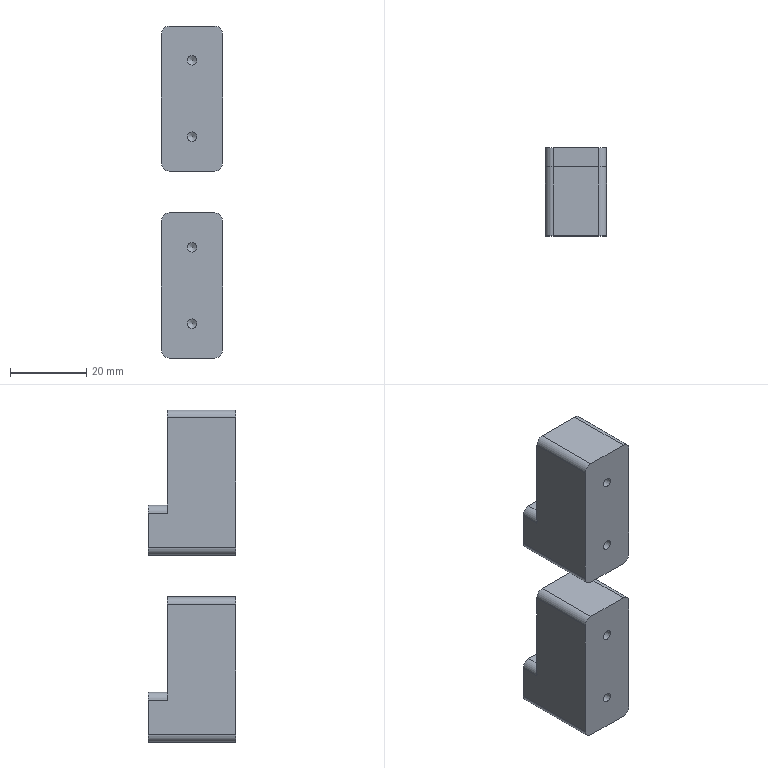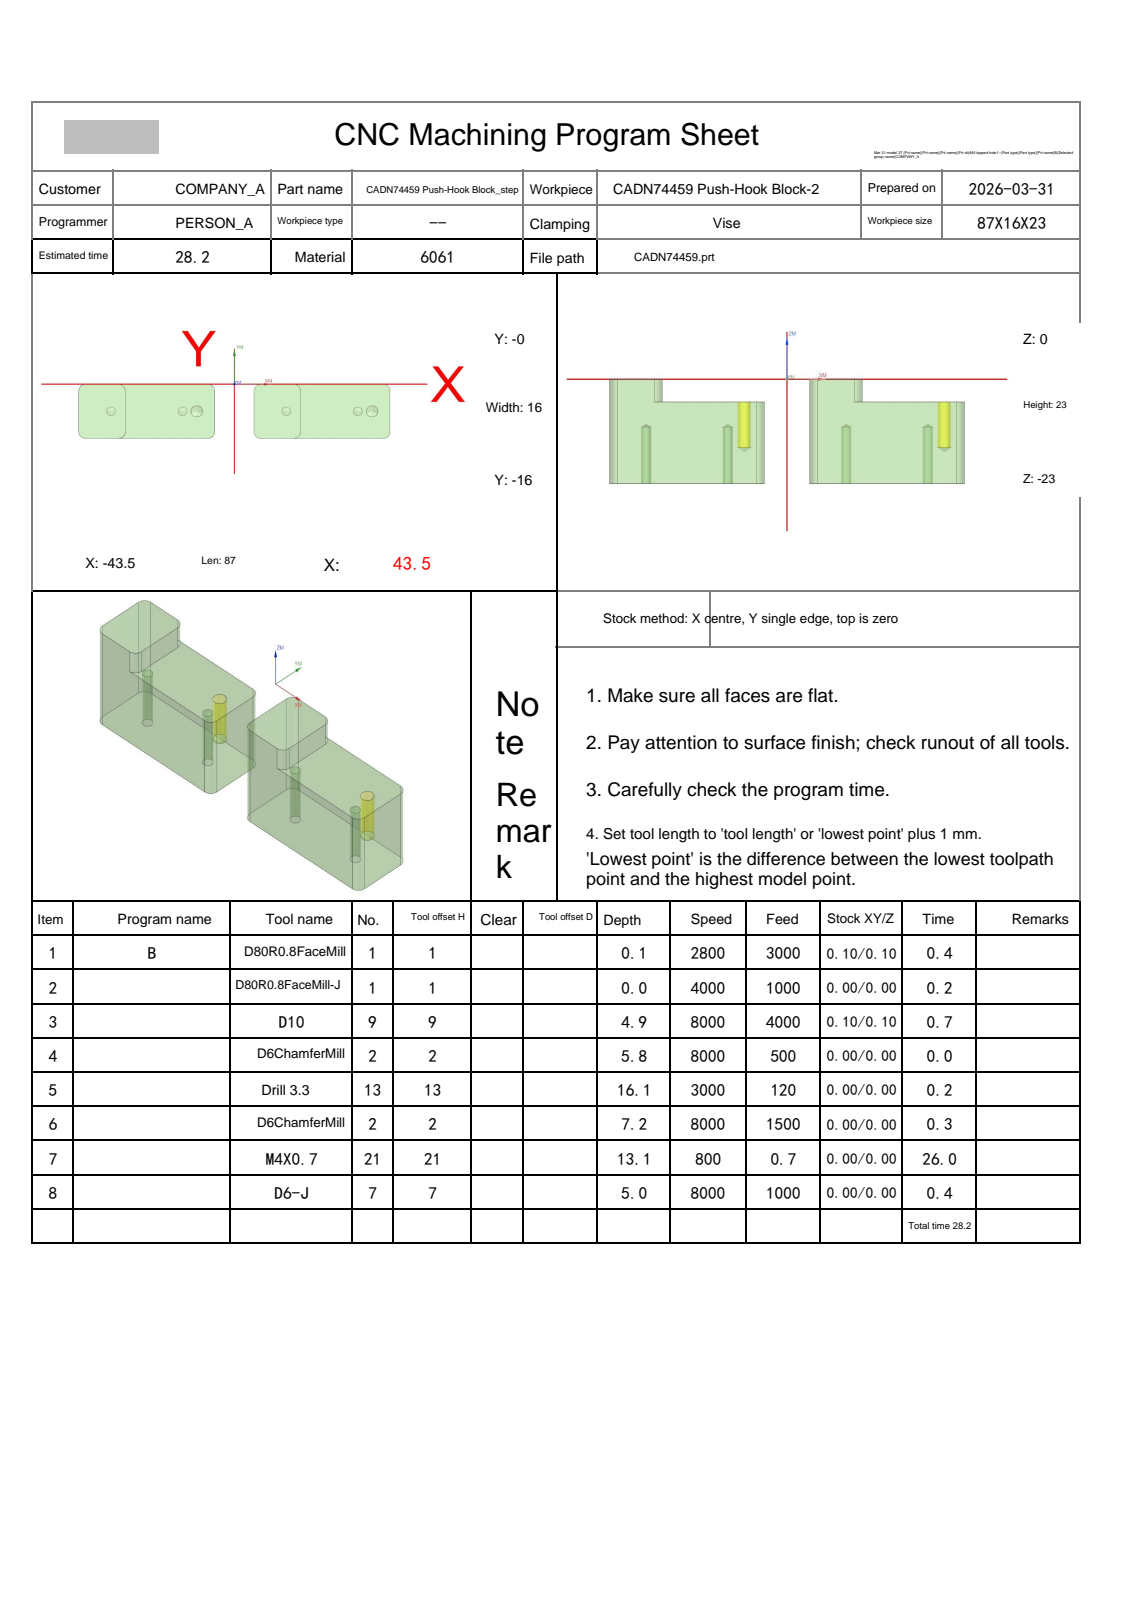NC program | NX | posted by the shop | part box 16 x 23 x 87 mm
Whole program:
%
O0001
(Machine time: 52.96 MIN)
(===Total Tool:6===)
(T1=D80R0.8 Mill D=80.  R=0.8  D-  H01 Z=0.    )
(T9=D10     D=10.  R=0.   D-  H09 Z=-4.9  )
(T2=D6ChamferMill   D=6.   R=0.   D-  H02 Z=-7.2  )
(T13=Drill 3.3  D=3.3  DR_a=118 D-  H13 Z=-16.09)
(T21=M4X0.7 D=3.3  DR_a=180 D-  H21 Z=-13.1 )
(T7=D6-J    D=6.   R=0.   D7  H07 Z=-5.   )
G80 G90 G17 G49 G40
G91 G28 Z0
M01
N1 T01 M06
(D80R0.8 Mill  D=80. R=0.8 H=01 ce=0.10 di=0.10)
G00 G90 G54 X95.597 Y-8. M03 S2800
G43 H01 Z20.
M08
Z4.02
G01 Z2.02 F3000.
X83.597
X-83.597
X-95.597
Z4.02
G00 X95.597
Z3.54
G01 Z1.54
X83.597
X-83.597
X-95.597
Z3.54
G00 X95.597
Z3.06
G01 Z1.06
X83.597
X-83.597
X-95.597
Z3.06
G00 X95.597
Z2.58
G01 Z.58
X83.597
X-83.597
X-95.597
Z2.58
G00 Z20.
X95.597
Z2.1
G01 Z.1
X83.597
X-83.597
X-95.597
Z2.1
G00 Z20.
G91 G28 Z0.0
M05
M09
G91 G28 Z0.0
M01
N2 T01 M06
(D80R0.8 Mill-J  D=80. R=0.8 H=01 ce=0.00 di=0.00)
G00 G90 G54 X95.499 Y-8. M03 S4000
G43 H01 Z20.
M08
Z2.
G01 Z0.0 F1000.
X83.499
X-83.499
X-95.499
Z2.
G00 Z20.
G91 G28 Z0.0
M05
M09
G91 G28 Z0.0
M01
N3 T09 M06
(D10  D=10. R=0. H=09 ce=0.10 di=0.10)
G00 G90 G54 X-4.168 Y-23.429 M03 S8000
G43 H09 Z11.8
M08
Z.956
G01 Z-.544 F4000.
X-3.429 Y-19.571
G03 X-2.9 Y-14. I-29.071 J5.571
G01 Y-2.
G03 X-3.352 Y3.155 I-29.6 J0.0
X-3.801 Y3.824 I-.985 J-.174
X-7.5 Y4.9 I-3.699 J-5.824
G01 X-10.559
G03 X-11.259 Y4.2 I0.0 J-.7
G01 X-11.233 Y4.01
G02 X-10.4 Y-2. I-21.267 J-6.01
G01 Y-14.
G02 X-11.282 Y-20.18 I-22.1 J0.0
X-12.241 Y-20.9 I-.96 J.28
G01 X-18.667
G02 X-19.267 Y-20.3 I0.0 J.6
X-19.213 Y-20.052 I.6 J0.0
G03 X-17.9 Y-14. I-13.287 J6.052
G01 Y-2.
G03 X-19.4 Y4.446 I-14.6 J0.0
X-20.118 Y4.988 I-.897 J-.442
G01 X-30.412 Y6.856
X-30.591 Y6.872
G03 X-31.591 Y5.872 I0.0 J-1.
X-30.827 Y4.9 I1. J0.0
G02 X-25.4 Y-2. I-1.673 J-6.9
G01 Y-14.
G02 X-30.827 Y-20.9 I-7.1 J0.0
G01 X-33.742 Y-21.607
Y-24.1
Z.956
G00 X-4.168 Y-23.429
Z.411
G01 Z-1.089
X-3.429 Y-19.571
G03 X-2.9 Y-14. I-29.071 J5.571
G01 Y-2.
G03 X-3.352 Y3.155 I-29.6 J0.0
X-3.801 Y3.824 I-.985 J-.174
X-7.5 Y4.9 I-3.699 J-5.824
G01 X-10.559
G03 X-11.259 Y4.2 I0.0 J-.7
G01 X-11.233 Y4.01
G02 X-10.4 Y-2. I-21.267 J-6.01
G01 Y-14.
G02 X-11.282 Y-20.18 I-22.1 J0.0
X-12.241 Y-20.9 I-.96 J.28
G01 X-18.667
G02 X-19.267 Y-20.3 I0.0 J.6
X-19.213 Y-20.052 I.6 J0.0
G03 X-17.9 Y-14. I-13.287 J6.052
G01 Y-2.
G03 X-19.4 Y4.446 I-14.6 J0.0
X-20.118 Y4.988 I-.897 J-.442
G01 X-30.412 Y6.856
X-30.591 Y6.872
G03 X-31.591 Y5.872 I0.0 J-1.
X-30.827 Y4.9 I1. J0.0
G02 X-25.4 Y-2. I-1.673 J-6.9
G01 Y-14.
G02 X-30.827 Y-20.9 I-7.1 J0.0
G01 X-33.742 Y-21.607
Y-24.1
Z.411
G00 X-4.168 Y-23.429
Z-.133
G01 Z-1.633
X-3.429 Y-19.571
G03 X-2.9 Y-14. I-29.071 J5.571
G01 Y-2.
G03 X-3.352 Y3.155 I-29.6 J0.0
X-3.801 Y3.824 I-.985 J-.174
X-7.5 Y4.9 I-3.699 J-5.824
G01 X-10.559
G03 X-11.259 Y4.2 I0.0 J-.7
G01 X-11.233 Y4.01
G02 X-10.4 Y-2. I-21.267 J-6.01
G01 Y-14.
G02 X-11.282 Y-20.18 I-22.1 J0.0
X-12.241 Y-20.9 I-.96 J.28
G01 X-18.667
G02 X-19.267 Y-20.3 I0.0 J.6
X-19.213 Y-20.052 I.6 J0.0
G03 X-17.9 Y-14. I-13.287 J6.052
G01 Y-2.
G03 X-19.4 Y4.446 I-14.6 J0.0
X-20.118 Y4.988 I-.897 J-.442
G01 X-30.412 Y6.856
X-30.591 Y6.872
G03 X-31.591 Y5.872 I0.0 J-1.
X-30.827 Y4.9 I1. J0.0
G02 X-25.4 Y-2. I-1.673 J-6.9
G01 Y-14.
G02 X-30.827 Y-20.9 I-7.1 J0.0
G01 X-33.742 Y-21.607
Y-24.1
Z-.133
G00 X-4.168 Y-23.429
Z-.678
G01 Z-2.178
X-3.429 Y-19.571
G03 X-2.9 Y-14. I-29.071 J5.571
G01 Y-2.
G03 X-3.352 Y3.155 I-29.6 J0.0
X-3.801 Y3.824 I-.985 J-.174
X-7.5 Y4.9 I-3.699 J-5.824
G01 X-10.559
G03 X-11.259 Y4.2 I0.0 J-.7
G01 X-11.233 Y4.01
G02 X-10.4 Y-2. I-21.267 J-6.01
G01 Y-14.
G02 X-11.282 Y-20.18 I-22.1 J0.0
X-12.241 Y-20.9 I-.96 J.28
G01 X-18.667
G02 X-19.267 Y-20.3 I0.0 J.6
X-19.213 Y-20.052 I.6 J0.0
G03 X-17.9 Y-14. I-13.287 J6.052
G01 Y-2.
G03 X-19.4 Y4.446 I-14.6 J0.0
X-20.118 Y4.988 I-.897 J-.442
G01 X-30.412 Y6.856
X-30.591 Y6.872
G03 X-31.591 Y5.872 I0.0 J-1.
X-30.827 Y4.9 I1. J0.0
G02 X-25.4 Y-2. I-1.673 J-6.9
G01 Y-14.
G02 X-30.827 Y-20.9 I-7.1 J0.0
G01 X-33.742 Y-21.607
Y-24.1
Z-.678
G00 X-4.168 Y-23.429
Z-1.222
G01 Z-2.722
X-3.429 Y-19.571
G03 X-2.9 Y-14. I-29.071 J5.571
G01 Y-2.
G03 X-3.352 Y3.155 I-29.6 J0.0
X-3.801 Y3.824 I-.985 J-.174
X-7.5 Y4.9 I-3.699 J-5.824
G01 X-10.559
G03 X-11.259 Y4.2 I0.0 J-.7
G01 X-11.233 Y4.01
G02 X-10.4 Y-2. I-21.267 J-6.01
G01 Y-14.
G02 X-11.282 Y-20.18 I-22.1 J0.0
X-12.241 Y-20.9 I-.96 J.28
G01 X-18.667
G02 X-19.267 Y-20.3 I0.0 J.6
X-19.213 Y-20.052 I.6 J0.0
G03 X-17.9 Y-14. I-13.287 J6.052
G01 Y-2.
G03 X-19.4 Y4.446 I-14.6 J0.0
X-20.118 Y4.988 I-.897 J-.442
G01 X-30.412 Y6.856
X-30.591 Y6.872
G03 X-31.591 Y5.872 I0.0 J-1.
X-30.827 Y4.9 I1. J0.0
G02 X-25.4 Y-2. I-1.673 J-6.9
G01 Y-14.
G02 X-30.827 Y-20.9 I-7.1 J0.0
G01 X-33.742 Y-21.607
Y-24.1
Z-1.222
G00 X-4.168 Y-23.429
Z-1.767
G01 Z-3.267
X-3.429 Y-19.571
G03 X-2.9 Y-14. I-29.071 J5.571
G01 Y-2.
G03 X-3.352 Y3.155 I-29.6 J0.0
X-3.801 Y3.824 I-.985 J-.174
X-7.5 Y4.9 I-3.699 J-5.824
G01 X-10.559
G03 X-11.259 Y4.2 I0.0 J-.7
G01 X-11.233 Y4.01
G02 X-10.4 Y-2. I-21.267 J-6.01
G01 Y-14.
G02 X-11.282 Y-20.18 I-22.1 J0.0
X-12.241 Y-20.9 I-.96 J.28
G01 X-18.667
G02 X-19.267 Y-20.3 I0.0 J.6
X-19.213 Y-20.052 I.6 J0.0
G03 X-17.9 Y-14. I-13.287 J6.052
G01 Y-2.
G03 X-19.4 Y4.446 I-14.6 J0.0
X-20.118 Y4.988 I-.897 J-.442
G01 X-30.412 Y6.856
X-30.591 Y6.872
G03 X-31.591 Y5.872 I0.0 J-1.
X-30.827 Y4.9 I1. J0.0
G02 X-25.4 Y-2. I-1.673 J-6.9
G01 Y-14.
G02 X-30.827 Y-20.9 I-7.1 J0.0
G01 X-33.742 Y-21.607
Y-24.1
Z-1.767
G00 X-4.168 Y-23.429
Z-2.311
G01 Z-3.811
X-3.429 Y-19.571
G03 X-2.9 Y-14. I-29.071 J5.571
G01 Y-2.
G03 X-3.352 Y3.155 I-29.6 J0.0
X-3.801 Y3.824 I-.985 J-.174
X-7.5 Y4.9 I-3.699 J-5.824
G01 X-10.559
G03 X-11.259 Y4.2 I0.0 J-.7
G01 X-11.233 Y4.01
G02 X-10.4 Y-2. I-21.267 J-6.01
G01 Y-14.
G02 X-11.282 Y-20.18 I-22.1 J0.0
X-12.241 Y-20.9 I-.96 J.28
G01 X-18.667
G02 X-19.267 Y-20.3 I0.0 J.6
X-19.213 Y-20.052 I.6 J0.0
G03 X-17.9 Y-14. I-13.287 J6.052
G01 Y-2.
G03 X-19.4 Y4.446 I-14.6 J0.0
X-20.118 Y4.988 I-.897 J-.442
G01 X-30.412 Y6.856
X-30.591 Y6.872
G03 X-31.591 Y5.872 I0.0 J-1.
X-30.827 Y4.9 I1. J0.0
G02 X-25.4 Y-2. I-1.673 J-6.9
G01 Y-14.
G02 X-30.827 Y-20.9 I-7.1 J0.0
G01 X-33.742 Y-21.607
Y-24.1
Z-2.311
G00 X-4.168 Y-23.429
Z-2.856
G01 Z-4.356
X-3.429 Y-19.571
G03 X-2.9 Y-14. I-29.071 J5.571
G01 Y-2.
G03 X-3.352 Y3.155 I-29.6 J0.0
X-3.801 Y3.824 I-.985 J-.174
X-7.5 Y4.9 I-3.699 J-5.824
G01 X-10.559
G03 X-11.259 Y4.2 I0.0 J-.7
G01 X-11.233 Y4.01
G02 X-10.4 Y-2. I-21.267 J-6.01
G01 Y-14.
G02 X-11.282 Y-20.18 I-22.1 J0.0
X-12.241 Y-20.9 I-.96 J.28
G01 X-18.667
G02 X-19.267 Y-20.3 I0.0 J.6
X-19.213 Y-20.052 I.6 J0.0
G03 X-17.9 Y-14. I-13.287 J6.052
G01 Y-2.
G03 X-19.4 Y4.446 I-14.6 J0.0
X-20.118 Y4.988 I-.897 J-.442
G01 X-30.412 Y6.856
X-30.591 Y6.872
G03 X-31.591 Y5.872 I0.0 J-1.
X-30.827 Y4.9 I1. J0.0
G02 X-25.4 Y-2. I-1.673 J-6.9
G01 Y-14.
G02 X-30.827 Y-20.9 I-7.1 J0.0
G01 X-33.742 Y-21.607
Y-24.1
Z-2.856
G00 X-4.168 Y-23.429
Z-3.4
G01 Z-4.9
X-3.429 Y-19.571
G03 X-2.9 Y-14. I-29.071 J5.571
G01 Y-2.
G03 X-3.352 Y3.155 I-29.6 J0.0
X-3.801 Y3.824 I-.985 J-.174
X-7.5 Y4.9 I-3.699 J-5.824
G01 X-10.559
G03 X-11.259 Y4.2 I0.0 J-.7
G01 X-11.233 Y4.01
G02 X-10.4 Y-2. I-21.267 J-6.01
G01 Y-14.
G02 X-11.282 Y-20.18 I-22.1 J0.0
X-12.241 Y-20.9 I-.96 J.28
G01 X-18.667
G02 X-19.267 Y-20.3 I0.0 J.6
X-19.213 Y-20.052 I.6 J0.0
G03 X-17.9 Y-14. I-13.287 J6.052
G01 Y-2.
G03 X-19.4 Y4.446 I-14.6 J0.0
X-20.118 Y4.988 I-.897 J-.442
G01 X-30.412 Y6.856
X-30.591 Y6.872
G03 X-31.591 Y5.872 I0.0 J-1.
X-30.827 Y4.9 I1. J0.0
G02 X-25.4 Y-2. I-1.673 J-6.9
G01 Y-14.
G02 X-30.827 Y-20.9 I-7.1 J0.0
G01 X-33.742 Y-21.607
Y-24.1
Z-3.4
G00 Z3.
X44.832 Y-23.429
Z.956
G01 Z-.544
X45.571 Y-19.571
G03 X46.1 Y-14. I-29.071 J5.571
G01 Y-2.
G03 X45.648 Y3.155 I-29.6 J0.0
X45.199 Y3.824 I-.985 J-.174
X41.5 Y4.9 I-3.699 J-5.824
G01 X38.441
G03 X37.741 Y4.2 I0.0 J-.7
G01 X37.767 Y4.01
G02 X38.6 Y-2. I-21.267 J-6.01
G01 Y-14.
G02 X37.718 Y-20.18 I-22.1 J0.0
X36.759 Y-20.9 I-.96 J.28
G01 X30.333
G02 X29.733 Y-20.3 I0.0 J.6
X29.787 Y-20.052 I.6 J0.0
G03 X31.1 Y-14. I-13.287 J6.052
G01 Y-2.
G03 X29.6 Y4.446 I-14.6 J0.0
X28.882 Y4.988 I-.897 J-.442
G01 X18.588 Y6.856
X18.409 Y6.872
G03 X17.409 Y5.872 I0.0 J-1.
X18.173 Y4.9 I1. J0.0
G02 X23.6 Y-2. I-1.673 J-6.9
G01 Y-14.
G02 X18.173 Y-20.9 I-7.1 J0.0
G01 X15.258 Y-21.607
Y-24.1
Z.956
G00 X44.832 Y-23.429
Z.411
G01 Z-1.089
X45.571 Y-19.571
G03 X46.1 Y-14. I-29.071 J5.571
G01 Y-2.
G03 X45.648 Y3.155 I-29.6 J0.0
X45.199 Y3.824 I-.985 J-.174
X41.5 Y4.9 I-3.699 J-5.824
G01 X38.441
G03 X37.741 Y4.2 I0.0 J-.7
G01 X37.767 Y4.01
G02 X38.6 Y-2. I-21.267 J-6.01
G01 Y-14.
G02 X37.718 Y-20.18 I-22.1 J0.0
X36.759 Y-20.9 I-.96 J.28
G01 X30.333
G02 X29.733 Y-20.3 I0.0 J.6
X29.787 Y-20.052 I.6 J0.0
G03 X31.1 Y-14. I-13.287 J6.052
G01 Y-2.
G03 X29.6 Y4.446 I-14.6 J0.0
X28.882 Y4.988 I-.897 J-.442
G01 X18.588 Y6.856
X18.409 Y6.872
G03 X17.409 Y5.872 I0.0 J-1.
X18.173 Y4.9 I1. J0.0
G02 X23.6 Y-2. I-1.673 J-6.9
G01 Y-14.
G02 X18.173 Y-20.9 I-7.1 J0.0
G01 X15.258 Y-21.607
Y-24.1
Z.411
G00 X44.832 Y-23.429
Z-.133
G01 Z-1.633
X45.571 Y-19.571
G03 X46.1 Y-14. I-29.071 J5.571
G01 Y-2.
G03 X45.648 Y3.155 I-29.6 J0.0
X45.199 Y3.824 I-.985 J-.174
X41.5 Y4.9 I-3.699 J-5.824
G01 X38.441
G03 X37.741 Y4.2 I0.0 J-.7
G01 X37.767 Y4.01
G02 X38.6 Y-2. I-21.267 J-6.01
G01 Y-14.
G02 X37.718 Y-20.18 I-22.1 J0.0
X36.759 Y-20.9 I-.96 J.28
G01 X30.333
G02 X29.733 Y-20.3 I0.0 J.6
X29.787 Y-20.052 I.6 J0.0
G03 X31.1 Y-14. I-13.287 J6.052
G01 Y-2.
G03 X29.6 Y4.446 I-14.6 J0.0
X28.882 Y4.988 I-.897 J-.442
G01 X18.588 Y6.856
X18.409 Y6.872
G03 X17.409 Y5.872 I0.0 J-1.
X18.173 Y4.9 I1. J0.0
G02 X23.6 Y-2. I-1.673 J-6.9
G01 Y-14.
G02 X18.173 Y-20.9 I-7.1 J0.0
G01 X15.258 Y-21.607
Y-24.1
Z-.133
G00 X44.832 Y-23.429
Z-.678
G01 Z-2.178
X45.571 Y-19.571
G03 X46.1 Y-14. I-29.071 J5.571
G01 Y-2.
G03 X45.648 Y3.155 I-29.6 J0.0
X45.199 Y3.824 I-.985 J-.174
X41.5 Y4.9 I-3.699 J-5.824
G01 X38.441
G03 X37.741 Y4.2 I0.0 J-.7
G01 X37.767 Y4.01
G02 X38.6 Y-2. I-21.267 J-6.01
G01 Y-14.
G02 X37.718 Y-20.18 I-22.1 J0.0
X36.759 Y-20.9 I-.96 J.28
G01 X30.333
G02 X29.733 Y-20.3 I0.0 J.6
X29.787 Y-20.052 I.6 J0.0
G03 X31.1 Y-14. I-13.287 J6.052
G01 Y-2.
G03 X29.6 Y4.446 I-14.6 J0.0
X28.882 Y4.988 I-.897 J-.442
G01 X18.588 Y6.856
X18.409 Y6.872
G03 X17.409 Y5.872 I0.0 J-1.
X18.173 Y4.9 I1. J0.0
G02 X23.6 Y-2. I-1.673 J-6.9
G01 Y-14.
G02 X18.173 Y-20.9 I-7.1 J0.0
G01 X15.258 Y-21.607
Y-24.1
Z-.678
G00 X44.832 Y-23.429
Z-1.222
G01 Z-2.722
X45.571 Y-19.571
G03 X46.1 Y-14. I-29.071 J5.571
G01 Y-2.
G03 X45.648 Y3.155 I-29.6 J0.0
X45.199 Y3.824 I-.985 J-.174
X41.5 Y4.9 I-3.699 J-5.824
G01 X38.441
G03 X37.741 Y4.2 I0.0 J-.7
G01 X37.767 Y4.01
G02 X38.6 Y-2. I-21.267 J-6.01
G01 Y-14.
G02 X37.718 Y-20.18 I-22.1 J0.0
X36.759 Y-20.9 I-.96 J.28
G01 X30.333
G02 X29.733 Y-20.3 I0.0 J.6
X29.787 Y-20.052 I.6 J0.0
G03 X31.1 Y-14. I-13.287 J6.052
G01 Y-2.
G03 X29.6 Y4.446 I-14.6 J0.0
X28.882 Y4.988 I-.897 J-.442
G01 X18.588 Y6.856
X18.409 Y6.872
G03 X17.409 Y5.872 I0.0 J-1.
X18.173 Y4.9 I1. J0.0
G02 X23.6 Y-2. I-1.673 J-6.9
G01 Y-14.
G02 X18.173 Y-20.9 I-7.1 J0.0
G01 X15.258 Y-21.607
Y-24.1
Z-1.222
G00 X44.832 Y-23.429
Z-1.767
G01 Z-3.267
X45.571 Y-19.571
G03 X46.1 Y-14. I-29.071 J5.571
G01 Y-2.
G03 X45.648 Y3.155 I-29.6 J0.0
X45.199 Y3.824 I-.985 J-.174
X41.5 Y4.9 I-3.699 J-5.824
G01 X38.441
G03 X37.741 Y4.2 I0.0 J-.7
G01 X37.767 Y4.01
G02 X38.6 Y-2. I-21.267 J-6.01
G01 Y-14.
G02 X37.718 Y-20.18 I-22.1 J0.0
X36.759 Y-20.9 I-.96 J.28
G01 X30.333
G02 X29.733 Y-20.3 I0.0 J.6
X29.787 Y-20.052 I.6 J0.0
G03 X31.1 Y-14. I-13.287 J6.052
G01 Y-2.
G03 X29.6 Y4.446 I-14.6 J0.0
X28.882 Y4.988 I-.897 J-.442
G01 X18.588 Y6.856
X18.409 Y6.872
G03 X17.409 Y5.872 I0.0 J-1.
X18.173 Y4.9 I1. J0.0
G02 X23.6 Y-2. I-1.673 J-6.9
G01 Y-14.
G02 X18.173 Y-20.9 I-7.1 J0.0
G01 X15.258 Y-21.607
Y-24.1
Z-1.767
G00 X44.832 Y-23.429
Z-2.311
G01 Z-3.811
X45.571 Y-19.571
G03 X46.1 Y-14. I-29.071 J5.571
G01 Y-2.
G03 X45.648 Y3.155 I-29.6 J0.0
X45.199 Y3.824 I-.985 J-.174
X41.5 Y4.9 I-3.699 J-5.824
G01 X38.441
G03 X37.741 Y4.2 I0.0 J-.7
G01 X37.767 Y4.01
G02 X38.6 Y-2. I-21.267 J-6.01
G01 Y-14.
G02 X37.718 Y-20.18 I-22.1 J0.0
X36.759 Y-20.9 I-.96 J.28
G01 X30.333
G02 X29.733 Y-20.3 I0.0 J.6
X29.787 Y-20.052 I.6 J0.0
G03 X31.1 Y-14. I-13.287 J6.052
G01 Y-2.
G03 X29.6 Y4.446 I-14.6 J0.0
X28.882 Y4.988 I-.897 J-.442
G01 X18.588 Y6.856
X18.409 Y6.872
G03 X17.409 Y5.872 I0.0 J-1.
X18.173 Y4.9 I1. J0.0
G02 X23.6 Y-2. I-1.673 J-6.9
G01 Y-14.
G02 X18.173 Y-20.9 I-7.1 J0.0
G01 X15.258 Y-21.607
Y-24.1
Z-2.311
G00 X44.832 Y-23.429
Z-2.856
G01 Z-4.356
X45.571 Y-19.571
G03 X46.1 Y-14. I-29.071 J5.571
G01 Y-2.
G03 X45.648 Y3.155 I-29.6 J0.0
X45.199 Y3.824 I-.985 J-.174
X41.5 Y4.9 I-3.699 J-5.824
G01 X38.441
G03 X37.741 Y4.2 I0.0 J-.7
G01 X37.767 Y4.01
G02 X38.6 Y-2. I-21.267 J-6.01
G01 Y-14.
G02 X37.718 Y-20.18 I-22.1 J0.0
X36.759 Y-20.9 I-.96 J.28
G01 X30.333
G02 X29.733 Y-20.3 I0.0 J.6
X29.787 Y-20.052 I.6 J0.0
G03 X31.1 Y-14. I-13.287 J6.052
G01 Y-2.
G03 X29.6 Y4.446 I-14.6 J0.0
X28.882 Y4.988 I-.897 J-.442
G01 X18.588 Y6.856
X18.409 Y6.872
G03 X17.409 Y5.872 I0.0 J-1.
X18.173 Y4.9 I1. J0.0
G02 X23.6 Y-2. I-1.673 J-6.9
G01 Y-14.
G02 X18.173 Y-20.9 I-7.1 J0.0
G01 X15.258 Y-21.607
Y-24.1
Z-2.856
G00 X44.832 Y-23.429
Z-3.4
G01 Z-4.9
X45.571 Y-19.571
G03 X46.1 Y-14. I-29.071 J5.571
G01 Y-2.
G03 X45.648 Y3.155 I-29.6 J0.0
X45.199 Y3.824 I-.985 J-.174
X41.5 Y4.9 I-3.699 J-5.824
G01 X38.441
G03 X37.741 Y4.2 I0.0 J-.7
G01 X37.767 Y4.01
G02 X38.6 Y-2. I-21.267 J-6.01
G01 Y-14.
G02 X37.718 Y-20.18 I-22.1 J0.0
X36.759 Y-20.9 I-.96 J.28
G01 X30.333
G02 X29.733 Y-20.3 I0.0 J.6
X29.787 Y-20.052 I.6 J0.0
G03 X31.1 Y-14. I-13.287 J6.052
G01 Y-2.
G03 X29.6 Y4.446 I-14.6 J0.0
X28.882 Y4.988 I-.897 J-.442
G01 X18.588 Y6.856
X18.409 Y6.872
G03 X17.409 Y5.872 I0.0 J-1.
X18.173 Y4.9 I1. J0.0
G02 X23.6 Y-2. I-1.673 J-6.9
G01 Y-14.
G02 X18.173 Y-20.9 I-7.1 J0.0
G01 X15.258 Y-21.607
Y-24.1
Z-3.4
G00 Z11.8
G91 G28 Z0.0
M05
M09
G91 G28 Z0.0
M01
N4 T02 M06
(D6ChamferMill  D=6. R=0. H=02 ce=0.00 di=0.10)
G00 G90 G54 X-10.5 Y-8. M03 S8000
G43 H02 Z20.
M08
G98 G81 X-10.5 Y-8. Z-5.8 R-4. F500.
X38.5
G80
G00 Z20.
G91 G28 Z0.0
M05
M09
G91 G28 Z0.0
M01
N5 T13 M06
(Drill 3.3 D=3.3 DR_a=118 H=13)
G00 G90 G54 X-10.5 Y-8. M03 S3000
G43 H13 Z20.
M08
G98 G83 X-10.5 Y-8. Z-16.091 R-4. F120. Q2.
X38.5
G80
G00 Z20.
G91 G28 Z0.0
M05
M09
G91 G28 Z0.0
M01
N6 T02 M06
(D6ChamferMill  D=6. R=0. H=02 ce=0.00 di=0.10)
G00 G90 G54 X-10.5 Y-8. M03 S8000
G43 H02 Z20.
M08
G98 G81 X-10.5 Y-8. Z-7.2 R-2. F500.
X38.5
G80
G00 Z20.
G00 G90 X4.273 Y-8.386 M03 S6500
Z20.
Z.172
G01 Z-1.2 F1500.
G03 X4.473 Y-8.1 I-1.532 J1.286
G01 X4.503 Y-8.054
X4.5 Y-8.
Y-2.
G02 X7.5 Y1. I3. J0.0
G01 X16.5
G02 X19.5 Y-2. I0.0 J-3.
G01 Y-14.
G02 X16.5 Y-17. I-3. J0.0
G01 X7.5
G02 X4.5 Y-14. I0.0 J3.
G01 Y-8.
X4.503 Y-7.946
X4.473 Y-7.9
G03 X4.273 Y-7.614 I-1.732 J-1.
G01 Z.172
G00 Z10.
X-29.273
Z.172
G01 Z-1.2
G03 X-29.473 Y-7.9 I1.532 J-1.286
G01 X-29.503 Y-7.946
X-29.5 Y-8.
Y-14.
G02 X-32.5 Y-17. I-3. J0.0
G01 X-41.5
G02 X-44.5 Y-14. I0.0 J3.
G01 Y-2.
G02 X-41.5 Y1. I3. J0.0
G01 X-32.5
G02 X-29.5 Y-2. I0.0 J-3.
G01 Y-8.
X-29.503 Y-8.054
X-29.473 Y-8.1
G03 X-29.273 Y-8.386 I1.732 J1.
G01 Z.172
G00 Z2.55
X-28.347 Y1.113
Z-1.796
G01 Z-6.2
X-28.284 Y1.052
X-28.204 Y1.013
X-28.183 Y.994
X-28.154 Y1.
X-7.5
G02 X-4.5 Y-2. I0.0 J-3.
G01 Y-14.
G02 X-7.5 Y-17. I-3. J0.0
G01 X-28.154
X-28.183 Y-16.994
X-28.204 Y-17.013
X-28.284 Y-17.052
X-28.347 Y-17.113
Z-1.796
G00 Z10.
X-10.006 Y-8.419
Z-4.595
G01 Z-6.2
G03 X-9.859 Y-8.103 I-1.732 J1.
G01 X-9.838 Y-8.053
X-9.85 Y-8.
G03 X-10.5 Y-7.35 I-.65 J0.0
X-11.15 Y-8. I0.0 J-.65
X-10.5 Y-8.65 I.65 J0.0
X-9.85 Y-8. I0.0 J.65
G01 X-9.838 Y-7.947
X-9.859 Y-7.897
G03 X-10.006 Y-7.581 I-1.879 J-.684
G01 Z-4.595
G00 Z10.
X20.653 Y1.113
Z-1.796
G01 Z-6.2
X20.716 Y1.052
X20.796 Y1.013
X20.817 Y.994
X20.846 Y1.
X41.5
G02 X44.5 Y-2. I0.0 J-3.
G01 Y-14.
G02 X41.5 Y-17. I-3. J0.0
G01 X20.846
X20.817 Y-16.994
X20.796 Y-17.013
X20.716 Y-17.052
X20.653 Y-17.113
Z-1.796
G00 Z10.
X38.994 Y-8.419
Z-4.595
G01 Z-6.2
G03 X39.141 Y-8.103 I-1.732 J1.
G01 X39.162 Y-8.053
X39.15 Y-8.
G03 X38.5 Y-7.35 I-.65 J0.0
X37.85 Y-8. I0.0 J-.65
X38.5 Y-8.65 I.65 J0.0
X39.15 Y-8. I0.0 J.65
G01 X39.162 Y-7.947
X39.141 Y-7.897
G03 X38.994 Y-7.581 I-1.879 J-.684
G01 Z-4.595
G00 Z20.
G91 G28 Z0.0
M05
M09
G91 G28 Z0.0
M01
N7 T21 M06
(M4X0.7 D=3.3 DR_a=180 H=21)
G00 G90 G54 X-10.5 Y-8. M03 S800
G43 H21 Z20.
M08
G95
G98 G84 X-10.5 Y-8. Z-13.1 R-4. F.7 Q3.
X38.5
G80
G94
G00 Z20.
G91 G28 Z0.0
M05
M09
G91 G28 Z0.0
M01
N8 T07 M06
(D6-J  D=6. R=0. H=07 ce=0.40 di=0.00)
G00 G90 G54 X-2.573 Y-17.764 M03 S8000
G43 H07 Z11.8
M08
Z-3.5
G01 Z-5. F1000.
X-5.103 Y-17.547
G02 X-6.2 Y-16.352 I.102 J1.196
G01 X-6.196 Y-16.249
G03 X-6.1 Y-14. I-26.304 J2.249
G01 Y-2.
G03 X-6.169 Y-.096 I-26.4 J0.0
X-6.547 Y.419 I-.598 J-.043
X-7.5 Y.6 I-.953 J-2.419
G01 X-8.649
G03 X-9.189 Y.06 I0.0 J-.54
G01 X-9.187 Y.014
G02 X-9.1 Y-2. I-23.313 J-2.014
G01 Y-14.
G02 X-9.19 Y-16.053 I-23.4 J0.0
X-9.788 Y-16.6 I-.598 J.053
G01 X-11.728
G02 X-12.208 Y-16.12 I0.0 J.48
G01 X-12.205 Y-16.071
G03 X-12.1 Y-14. I-20.295 J2.071
G01 Y-2.
G03 X-12.204 Y.061 I-20.4 J0.0
X-12.801 Y.6 I-.597 J-.061
G01 X-14.746
G03 X-15.226 Y.12 I0.0 J-.48
G01 X-15.223 Y.063
G02 X-15.1 Y-2. I-17.277 J-2.063
G01 Y-14.
G02 X-15.224 Y-16.071 I-17.4 J0.0
X-15.819 Y-16.6 I-.596 J.071
G01 X-17.772
G02 X-18.252 Y-16.12 I0.0 J.48
G01 X-18.247 Y-16.052
G03 X-18.1 Y-14. I-14.253 J2.052
G01 Y-2.
G03 X-18.252 Y.087 I-14.4 J0.0
X-18.846 Y.6 I-.594 J-.087
G01 X-20.811
G03 X-21.291 Y.12 I0.0 J-.48
G01 X-21.283 Y.035
G02 X-21.1 Y-2. I-11.217 J-2.035
G01 Y-14.
G02 X-21.297 Y-16.111 I-11.4 J0.0
X-21.887 Y-16.6 I-.59 J.111
G01 X-23.954
G02 X-24.374 Y-16.18 I0.0 J.42
G01 X-24.361 Y-16.076
G03 X-24.1 Y-14. I-8.139 J2.076
G01 Y-2.
G03 X-24.419 Y.294 I-8.4 J0.0
X-24.804 Y.699 I-.577 J-.164
G01 X-27.049 Y1.457
X-27.241 Y1.489
G03 X-27.841 Y.889 I0.0 J-.6
X-27.767 Y.6 I.6 J0.0
G02 X-27.1 Y-2. I-4.733 J-2.6
G01 Y-14.
G02 X-27.767 Y-16.6 I-5.4 J0.0
G03 X-27.915 Y-17.178 I1.052 J-.578
X-27.293 Y-18.23 I1.2 J0.0
G01 X-23.706 Y-20.2
Z-3.5
G00 Z11.8
X46.427 Y-17.764
Z-3.5
G01 Z-5.
X43.897 Y-17.547
G02 X42.8 Y-16.352 I.102 J1.196
G01 X42.804 Y-16.249
G03 X42.9 Y-14. I-26.304 J2.249
G01 Y-2.
G03 X42.831 Y-.096 I-26.4 J0.0
X42.453 Y.419 I-.598 J-.043
X41.5 Y.6 I-.953 J-2.419
G01 X40.351
G03 X39.811 Y.06 I0.0 J-.54
G01 X39.813 Y.014
G02 X39.9 Y-2. I-23.313 J-2.014
G01 Y-14.
G02 X39.81 Y-16.053 I-23.4 J0.0
X39.212 Y-16.6 I-.598 J.053
G01 X37.272
G02 X36.792 Y-16.12 I0.0 J.48
G01 X36.795 Y-16.072
G03 X36.9 Y-14. I-20.295 J2.072
G01 Y-2.
G03 X36.796 Y.061 I-20.4 J0.0
X36.199 Y.6 I-.597 J-.061
G01 X34.254
G03 X33.774 Y.12 I0.0 J-.48
G01 X33.777 Y.063
G02 X33.9 Y-2. I-17.277 J-2.063
G01 Y-14.
G02 X33.776 Y-16.071 I-17.4 J0.0
X33.181 Y-16.6 I-.596 J.071
G01 X31.228
G02 X30.748 Y-16.12 I0.0 J.48
G01 X30.753 Y-16.052
G03 X30.9 Y-14. I-14.253 J2.052
G01 Y-2.
G03 X30.748 Y.087 I-14.4 J0.0
X30.154 Y.6 I-.594 J-.087
G01 X28.189
G03 X27.709 Y.12 I0.0 J-.48
G01 X27.717 Y.035
G02 X27.9 Y-2. I-11.217 J-2.035
G01 Y-14.
G02 X27.703 Y-16.111 I-11.4 J0.0
X27.113 Y-16.6 I-.59 J.111
G01 X25.046
G02 X24.626 Y-16.18 I0.0 J.42
G01 X24.639 Y-16.076
G03 X24.9 Y-14. I-8.139 J2.076
G01 Y-2.
G03 X24.581 Y.294 I-8.4 J0.0
X24.196 Y.699 I-.577 J-.164
G01 X21.951 Y1.457
X21.759 Y1.489
G03 X21.159 Y.889 I0.0 J-.6
X21.233 Y.6 I.6 J0.0
G02 X21.9 Y-2. I-4.733 J-2.6
G01 Y-14.
G02 X21.233 Y-16.6 I-5.4 J0.0
G03 X21.085 Y-17.178 I1.052 J-.578
X21.707 Y-18.23 I1.2 J0.0
G01 X25.294 Y-20.2
Z-3.5
G00 Z11.8
G00 G90 X-33.485 Y4.4 M03 S8000
Z11.8
Z-4.
G01 Z-5. F1000.
G41 D07
Y4.2
Y4.196
G03 X-32.327 Y2.997 I1.2 J0.0
G02 X-27.5 Y-2. I-.173 J-4.997
G01 Y-14.
G02 X-32.327 Y-18.997 I-5. J0.0
G03 X-33.485 Y-20.196 I.042 J-1.199
G01 Y-20.2
G40 Y-20.4
Z-4.
G00 Z11.8
X15.515 Y4.4
Z-4.
G01 Z-5.
G41 D07
Y4.2
Y4.196
G03 X16.673 Y2.997 I1.2 J0.0
G02 X21.5 Y-2. I-.173 J-4.997
G01 Y-14.
G02 X16.673 Y-18.997 I-5. J0.0
G03 X15.515 Y-20.196 I.042 J-1.199
G01 Y-20.2
G40 Y-20.4
Z-4.
G00 Z11.8
M05
M09
G91 G28 Z0.0
G91 G28 Y0.0
M30
%